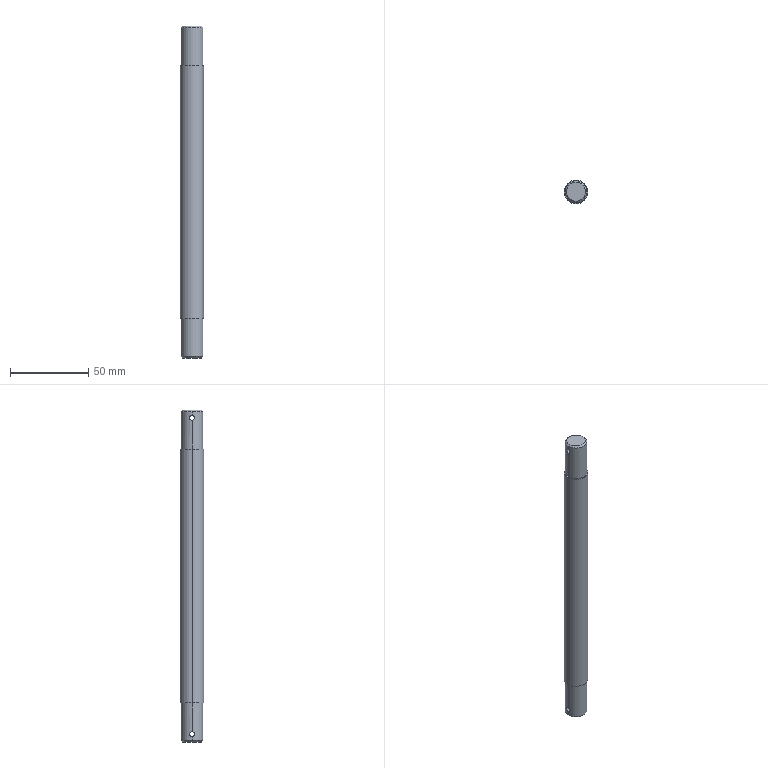Part | SolidWorks | features Chamfer 1, ICE 1, Revolution 1 | 1 solid | 18 faces | box 15 x 15 x 212 mm | volume 36086 mm3 | cylinder 10 | cone 4 | plane 4 | commonest cylinder face diameters 3 x4 14 x4 15 x2
STEP:
#1=CARTESIAN_POINT('',(6.,0.,0.));
#2=VERTEX_POINT('',#1);
#3=CARTESIAN_POINT('',(-6.,0.,0.));
#4=VERTEX_POINT('',#3);
#5=CARTESIAN_POINT('',(0.,0.,0.));
#6=DIRECTION('',(0.,0.,1.));
#7=DIRECTION('',(1.,0.,0.));
#8=AXIS2_PLACEMENT_3D('',#5,#6,#7);
#9=CIRCLE('',#8,6.);
#10=EDGE_CURVE('',#2,#4,#9,.T.);
#11=ORIENTED_EDGE('',*,*,#10,.F.);
#12=CARTESIAN_POINT('',(7.,0.,-1.));
#13=VERTEX_POINT('',#12);
#14=CARTESIAN_POINT('',(6.,0.,0.));
#15=DIRECTION('',(0.7071,0.,-0.7071));
#16=VECTOR('',#15,1000.);
#17=LINE('',#14,#16);
#18=EDGE_CURVE('',#2,#13,#17,.T.);
#19=ORIENTED_EDGE('',*,*,#18,.T.);
#20=CARTESIAN_POINT('',(-7.,0.,-1.));
#21=VERTEX_POINT('',#20);
#22=CARTESIAN_POINT('',(0.,0.,-1.));
#23=DIRECTION('',(0.,0.,-1.));
#24=DIRECTION('',(1.,0.,0.));
#25=AXIS2_PLACEMENT_3D('',#22,#23,#24);
#26=CIRCLE('',#25,7.);
#27=EDGE_CURVE('',#21,#13,#26,.T.);
#28=ORIENTED_EDGE('',*,*,#27,.F.);
#29=CARTESIAN_POINT('',(-6.,0.,0.));
#30=DIRECTION('',(-0.7071,0.,-0.7071));
#31=VECTOR('',#30,1000.);
#32=LINE('',#29,#31);
#33=EDGE_CURVE('',#4,#21,#32,.T.);
#34=ORIENTED_EDGE('',*,*,#33,.F.);
#35=EDGE_LOOP('',(#11,#19,#28,#34));
#36=FACE_OUTER_BOUND('',#35,.T.);
#37=CARTESIAN_POINT('',(0.,0.,0.));
#38=DIRECTION('',(0.,0.,-1.));
#39=DIRECTION('',(-1.,0.,0.));
#40=AXIS2_PLACEMENT_3D('',#37,#38,#39);
#41=CONICAL_SURFACE('',#40,6.,0.7854);
#42=ADVANCED_FACE('',(#36),#41,.T.);
#43=CARTESIAN_POINT('',(-6.,0.,-212.));
#44=VERTEX_POINT('',#43);
#45=CARTESIAN_POINT('',(6.,0.,-212.));
#46=VERTEX_POINT('',#45);
#47=CARTESIAN_POINT('',(0.,0.,-212.));
#48=DIRECTION('',(0.,0.,-1.));
#49=DIRECTION('',(1.,0.,0.));
#50=AXIS2_PLACEMENT_3D('',#47,#48,#49);
#51=CIRCLE('',#50,6.);
#52=EDGE_CURVE('',#44,#46,#51,.T.);
#53=ORIENTED_EDGE('',*,*,#52,.F.);
#54=CARTESIAN_POINT('',(-7.,0.,-211.));
#55=VERTEX_POINT('',#54);
#56=CARTESIAN_POINT('',(-7.,0.,-211.));
#57=DIRECTION('',(-0.7071,0.,0.7071));
#58=VECTOR('',#57,1000.);
#59=LINE('',#56,#58);
#60=EDGE_CURVE('',#44,#55,#59,.T.);
#61=ORIENTED_EDGE('',*,*,#60,.T.);
#62=CARTESIAN_POINT('',(7.,0.,-211.));
#63=VERTEX_POINT('',#62);
#64=CARTESIAN_POINT('',(0.,0.,-211.));
#65=DIRECTION('',(0.,0.,1.));
#66=DIRECTION('',(1.,0.,0.));
#67=AXIS2_PLACEMENT_3D('',#64,#65,#66);
#68=CIRCLE('',#67,7.);
#69=EDGE_CURVE('',#63,#55,#68,.T.);
#70=ORIENTED_EDGE('',*,*,#69,.F.);
#71=CARTESIAN_POINT('',(7.,0.,-211.));
#72=DIRECTION('',(0.7071,0.,0.7071));
#73=VECTOR('',#72,1000.);
#74=LINE('',#71,#73);
#75=EDGE_CURVE('',#46,#63,#74,.T.);
#76=ORIENTED_EDGE('',*,*,#75,.F.);
#77=EDGE_LOOP('',(#53,#61,#70,#76));
#78=FACE_OUTER_BOUND('',#77,.T.);
#79=CARTESIAN_POINT('',(0.,0.,-211.));
#80=DIRECTION('',(0.,0.,1.));
#81=DIRECTION('',(1.,0.,0.));
#82=AXIS2_PLACEMENT_3D('',#79,#80,#81);
#83=CONICAL_SURFACE('',#82,7.,0.7854);
#84=ADVANCED_FACE('',(#78),#83,.T.);
#85=CARTESIAN_POINT('',(-7.,0.,-208.5));
#86=VERTEX_POINT('',#85);
#87=CARTESIAN_POINT('',(-7.,0.,-205.5));
#88=VERTEX_POINT('',#87);
#89=CARTESIAN_POINT('',(-7.,0.,-208.5));
#90=CARTESIAN_POINT('',(-7.,-0.09942,-208.5));
#91=CARTESIAN_POINT('',(-6.998,-0.1971,-208.49));
#92=CARTESIAN_POINT('',(-6.99,-0.3892,-208.452));
#93=CARTESIAN_POINT('',(-6.984,-0.4847,-208.423));
#94=CARTESIAN_POINT('',(-6.969,-0.6662,-208.348));
#95=CARTESIAN_POINT('',(-6.96,-0.7523,-208.301));
#96=CARTESIAN_POINT('',(-6.94,-0.9151,-208.193));
#97=CARTESIAN_POINT('',(-6.93,-0.992,-208.129));
#98=CARTESIAN_POINT('',(-6.898,-1.199,-207.922));
#99=CARTESIAN_POINT('',(-6.877,-1.31,-207.755));
#100=CARTESIAN_POINT('',(-6.846,-1.46,-207.395));
#101=CARTESIAN_POINT('',(-6.837,-1.5,-207.197));
#102=CARTESIAN_POINT('',(-6.837,-1.5,-206.902));
#103=CARTESIAN_POINT('',(-6.84,-1.49,-206.803));
#104=CARTESIAN_POINT('',(-6.848,-1.452,-206.61));
#105=CARTESIAN_POINT('',(-6.854,-1.423,-206.516));
#106=CARTESIAN_POINT('',(-6.877,-1.31,-206.243));
#107=CARTESIAN_POINT('',(-6.898,-1.2,-206.078));
#108=CARTESIAN_POINT('',(-6.93,-0.9909,-205.87));
#109=CARTESIAN_POINT('',(-6.94,-0.9154,-205.808));
#110=CARTESIAN_POINT('',(-6.96,-0.7532,-205.699));
#111=CARTESIAN_POINT('',(-6.969,-0.6653,-205.652));
#112=CARTESIAN_POINT('',(-6.984,-0.4841,-205.577));
#113=CARTESIAN_POINT('',(-6.99,-0.3905,-205.548));
#114=CARTESIAN_POINT('',(-6.998,-0.1976,-205.51));
#115=CARTESIAN_POINT('',(-7.,-0.09806,-205.5));
#116=CARTESIAN_POINT('',(-7.,0.,-205.5));
#117=B_SPLINE_CURVE_WITH_KNOTS('',3,(#89,#90,#91,#92,#93,#94,#95,#96,#97,#98,#99,#100,#101,#102,#103,#104,#105,#106,#107,#108,#109,#110,#111,#112,#113,#114,#115,#116),.UNSPECIFIED.,.F.,.F.,(4,2,2,2,2,2,2,2,2,2,2,2,2,4),(0.,0.000294,0.0005879,0.0008819,0.001176,0.001764,0.002352,0.002646,0.00294,0.003528,0.003821,0.004115,0.004409,0.004703),.UNSPECIFIED.);
#118=EDGE_CURVE('',#86,#88,#117,.T.);
#119=ORIENTED_EDGE('',*,*,#118,.T.);
#120=CARTESIAN_POINT('',(7.,0.,-205.5));
#121=VERTEX_POINT('',#120);
#122=CARTESIAN_POINT('',(-7.5,0.,-205.5));
#123=DIRECTION('',(1.,0.,0.));
#124=VECTOR('',#123,1000.);
#125=LINE('',#122,#124);
#126=EDGE_CURVE('',#88,#121,#125,.T.);
#127=ORIENTED_EDGE('',*,*,#126,.T.);
#128=CARTESIAN_POINT('',(7.,0.,-208.5));
#129=VERTEX_POINT('',#128);
#130=CARTESIAN_POINT('',(7.,0.,-205.5));
#131=CARTESIAN_POINT('',(7.,-0.1961,-205.5));
#132=CARTESIAN_POINT('',(6.991,-0.394,-205.54));
#133=CARTESIAN_POINT('',(6.962,-0.7552,-205.689));
#134=CARTESIAN_POINT('',(6.94,-0.9218,-205.801));
#135=CARTESIAN_POINT('',(6.909,-1.129,-206.008));
#136=CARTESIAN_POINT('',(6.898,-1.192,-206.085));
#137=CARTESIAN_POINT('',(6.878,-1.301,-206.247));
#138=CARTESIAN_POINT('',(6.869,-1.347,-206.333));
#139=CARTESIAN_POINT('',(6.846,-1.461,-206.606));
#140=CARTESIAN_POINT('',(6.837,-1.5,-206.801));
#141=CARTESIAN_POINT('',(6.837,-1.5,-207.098));
#142=CARTESIAN_POINT('',(6.84,-1.49,-207.196));
#143=CARTESIAN_POINT('',(6.848,-1.452,-207.388));
#144=CARTESIAN_POINT('',(6.854,-1.423,-207.484));
#145=CARTESIAN_POINT('',(6.877,-1.311,-207.756));
#146=CARTESIAN_POINT('',(6.898,-1.199,-207.922));
#147=CARTESIAN_POINT('',(6.94,-0.9236,-208.198));
#148=CARTESIAN_POINT('',(6.961,-0.7569,-208.31));
#149=CARTESIAN_POINT('',(6.991,-0.396,-208.46));
#150=CARTESIAN_POINT('',(7.,-0.1988,-208.5));
#151=CARTESIAN_POINT('',(7.,0.,-208.5));
#152=B_SPLINE_CURVE_WITH_KNOTS('',3,(#130,#131,#132,#133,#134,#135,#136,#137,#138,#139,#140,#141,#142,#143,#144,#145,#146,#147,#148,#149,#150,#151),.UNSPECIFIED.,.F.,.F.,(4,2,2,2,2,2,2,2,2,2,4),(0.004703,0.005291,0.005879,0.006173,0.006467,0.007054,0.007348,0.007642,0.00823,0.008818,0.009405),.UNSPECIFIED.);
#153=EDGE_CURVE('',#121,#129,#152,.T.);
#154=ORIENTED_EDGE('',*,*,#153,.T.);
#155=CARTESIAN_POINT('',(-7.5,0.,-208.5));
#156=DIRECTION('',(1.,0.,0.));
#157=VECTOR('',#156,1000.);
#158=LINE('',#155,#157);
#159=EDGE_CURVE('',#86,#129,#158,.T.);
#160=ORIENTED_EDGE('',*,*,#159,.F.);
#161=EDGE_LOOP('',(#119,#127,#154,#160));
#162=FACE_OUTER_BOUND('',#161,.T.);
#163=CARTESIAN_POINT('',(-7.5,0.,-207.));
#164=DIRECTION('',(1.,0.,0.));
#165=DIRECTION('',(0.,0.,-1.));
#166=AXIS2_PLACEMENT_3D('',#163,#164,#165);
#167=CYLINDRICAL_SURFACE('',#166,1.5);
#168=ADVANCED_FACE('',(#162),#167,.F.);
#169=CARTESIAN_POINT('',(-7.,0.,-6.5));
#170=VERTEX_POINT('',#169);
#171=CARTESIAN_POINT('',(-7.,0.,-3.5));
#172=VERTEX_POINT('',#171);
#173=CARTESIAN_POINT('',(-7.,0.,-6.5));
#174=CARTESIAN_POINT('',(-7.,-0.09942,-6.5));
#175=CARTESIAN_POINT('',(-6.998,-0.1971,-6.49));
#176=CARTESIAN_POINT('',(-6.99,-0.3892,-6.452));
#177=CARTESIAN_POINT('',(-6.984,-0.4847,-6.423));
#178=CARTESIAN_POINT('',(-6.969,-0.6662,-6.348));
#179=CARTESIAN_POINT('',(-6.96,-0.7523,-6.301));
#180=CARTESIAN_POINT('',(-6.94,-0.9151,-6.193));
#181=CARTESIAN_POINT('',(-6.93,-0.992,-6.129));
#182=CARTESIAN_POINT('',(-6.898,-1.199,-5.922));
#183=CARTESIAN_POINT('',(-6.877,-1.31,-5.755));
#184=CARTESIAN_POINT('',(-6.846,-1.46,-5.395));
#185=CARTESIAN_POINT('',(-6.837,-1.5,-5.197));
#186=CARTESIAN_POINT('',(-6.837,-1.5,-4.902));
#187=CARTESIAN_POINT('',(-6.84,-1.49,-4.803));
#188=CARTESIAN_POINT('',(-6.848,-1.452,-4.61));
#189=CARTESIAN_POINT('',(-6.854,-1.423,-4.516));
#190=CARTESIAN_POINT('',(-6.877,-1.31,-4.243));
#191=CARTESIAN_POINT('',(-6.898,-1.2,-4.078));
#192=CARTESIAN_POINT('',(-6.93,-0.9909,-3.87));
#193=CARTESIAN_POINT('',(-6.94,-0.9154,-3.808));
#194=CARTESIAN_POINT('',(-6.96,-0.7532,-3.699));
#195=CARTESIAN_POINT('',(-6.969,-0.6653,-3.652));
#196=CARTESIAN_POINT('',(-6.984,-0.4841,-3.577));
#197=CARTESIAN_POINT('',(-6.99,-0.3905,-3.548));
#198=CARTESIAN_POINT('',(-6.998,-0.1976,-3.51));
#199=CARTESIAN_POINT('',(-7.,-0.09806,-3.5));
#200=CARTESIAN_POINT('',(-7.,0.,-3.5));
#201=B_SPLINE_CURVE_WITH_KNOTS('',3,(#173,#174,#175,#176,#177,#178,#179,#180,#181,#182,#183,#184,#185,#186,#187,#188,#189,#190,#191,#192,#193,#194,#195,#196,#197,#198,#199,#200),.UNSPECIFIED.,.F.,.F.,(4,2,2,2,2,2,2,2,2,2,2,2,2,4),(0.,0.000294,0.0005879,0.0008819,0.001176,0.001764,0.002352,0.002646,0.00294,0.003528,0.003821,0.004115,0.004409,0.004703),.UNSPECIFIED.);
#202=EDGE_CURVE('',#170,#172,#201,.T.);
#203=ORIENTED_EDGE('',*,*,#202,.T.);
#204=CARTESIAN_POINT('',(7.,0.,-3.5));
#205=VERTEX_POINT('',#204);
#206=CARTESIAN_POINT('',(-7.5,0.,-3.5));
#207=DIRECTION('',(1.,0.,0.));
#208=VECTOR('',#207,1000.);
#209=LINE('',#206,#208);
#210=EDGE_CURVE('',#172,#205,#209,.T.);
#211=ORIENTED_EDGE('',*,*,#210,.T.);
#212=CARTESIAN_POINT('',(7.,0.,-6.5));
#213=VERTEX_POINT('',#212);
#214=CARTESIAN_POINT('',(7.,0.,-3.5));
#215=CARTESIAN_POINT('',(7.,-0.1961,-3.5));
#216=CARTESIAN_POINT('',(6.991,-0.394,-3.54));
#217=CARTESIAN_POINT('',(6.962,-0.7552,-3.689));
#218=CARTESIAN_POINT('',(6.94,-0.9218,-3.801));
#219=CARTESIAN_POINT('',(6.909,-1.129,-4.008));
#220=CARTESIAN_POINT('',(6.898,-1.192,-4.085));
#221=CARTESIAN_POINT('',(6.878,-1.301,-4.247));
#222=CARTESIAN_POINT('',(6.869,-1.347,-4.333));
#223=CARTESIAN_POINT('',(6.846,-1.461,-4.606));
#224=CARTESIAN_POINT('',(6.837,-1.5,-4.801));
#225=CARTESIAN_POINT('',(6.837,-1.5,-5.098));
#226=CARTESIAN_POINT('',(6.84,-1.49,-5.196));
#227=CARTESIAN_POINT('',(6.848,-1.452,-5.388));
#228=CARTESIAN_POINT('',(6.854,-1.423,-5.484));
#229=CARTESIAN_POINT('',(6.877,-1.311,-5.756));
#230=CARTESIAN_POINT('',(6.898,-1.199,-5.922));
#231=CARTESIAN_POINT('',(6.94,-0.9236,-6.198));
#232=CARTESIAN_POINT('',(6.961,-0.7569,-6.31));
#233=CARTESIAN_POINT('',(6.991,-0.396,-6.46));
#234=CARTESIAN_POINT('',(7.,-0.1988,-6.5));
#235=CARTESIAN_POINT('',(7.,0.,-6.5));
#236=B_SPLINE_CURVE_WITH_KNOTS('',3,(#214,#215,#216,#217,#218,#219,#220,#221,#222,#223,#224,#225,#226,#227,#228,#229,#230,#231,#232,#233,#234,#235),.UNSPECIFIED.,.F.,.F.,(4,2,2,2,2,2,2,2,2,2,4),(0.004703,0.005291,0.005879,0.006173,0.006467,0.007054,0.007348,0.007642,0.00823,0.008818,0.009405),.UNSPECIFIED.);
#237=EDGE_CURVE('',#205,#213,#236,.T.);
#238=ORIENTED_EDGE('',*,*,#237,.T.);
#239=CARTESIAN_POINT('',(-7.5,0.,-6.5));
#240=DIRECTION('',(1.,0.,0.));
#241=VECTOR('',#240,1000.);
#242=LINE('',#239,#241);
#243=EDGE_CURVE('',#170,#213,#242,.T.);
#244=ORIENTED_EDGE('',*,*,#243,.F.);
#245=EDGE_LOOP('',(#203,#211,#238,#244));
#246=FACE_OUTER_BOUND('',#245,.T.);
#247=CARTESIAN_POINT('',(-7.5,0.,-5.));
#248=DIRECTION('',(1.,0.,0.));
#249=DIRECTION('',(0.,0.,-1.));
#250=AXIS2_PLACEMENT_3D('',#247,#248,#249);
#251=CYLINDRICAL_SURFACE('',#250,1.5);
#252=ADVANCED_FACE('',(#246),#251,.F.);
#253=CARTESIAN_POINT('',(7.,0.,-25.));
#254=VERTEX_POINT('',#253);
#255=CARTESIAN_POINT('',(-7.,0.,-25.));
#256=VERTEX_POINT('',#255);
#257=CARTESIAN_POINT('',(0.,0.,-25.));
#258=DIRECTION('',(0.,0.,1.));
#259=DIRECTION('',(1.,0.,0.));
#260=AXIS2_PLACEMENT_3D('',#257,#258,#259);
#261=CIRCLE('',#260,7.);
#262=EDGE_CURVE('',#254,#256,#261,.T.);
#263=ORIENTED_EDGE('',*,*,#262,.T.);
#264=CARTESIAN_POINT('',(-7.,0.,-25.));
#265=DIRECTION('',(0.,0.,1.));
#266=VECTOR('',#265,1000.);
#267=LINE('',#264,#266);
#268=EDGE_CURVE('',#256,#170,#267,.T.);
#269=ORIENTED_EDGE('',*,*,#268,.T.);
#270=CARTESIAN_POINT('',(-7.,0.,-3.5));
#271=CARTESIAN_POINT('',(-7.,0.1961,-3.5));
#272=CARTESIAN_POINT('',(-6.991,0.394,-3.54));
#273=CARTESIAN_POINT('',(-6.962,0.7552,-3.689));
#274=CARTESIAN_POINT('',(-6.94,0.9218,-3.801));
#275=CARTESIAN_POINT('',(-6.909,1.129,-4.008));
#276=CARTESIAN_POINT('',(-6.898,1.192,-4.085));
#277=CARTESIAN_POINT('',(-6.878,1.301,-4.247));
#278=CARTESIAN_POINT('',(-6.869,1.347,-4.333));
#279=CARTESIAN_POINT('',(-6.846,1.461,-4.606));
#280=CARTESIAN_POINT('',(-6.837,1.5,-4.801));
#281=CARTESIAN_POINT('',(-6.837,1.5,-5.098));
#282=CARTESIAN_POINT('',(-6.84,1.49,-5.196));
#283=CARTESIAN_POINT('',(-6.848,1.452,-5.388));
#284=CARTESIAN_POINT('',(-6.854,1.423,-5.484));
#285=CARTESIAN_POINT('',(-6.877,1.311,-5.756));
#286=CARTESIAN_POINT('',(-6.898,1.199,-5.922));
#287=CARTESIAN_POINT('',(-6.94,0.9236,-6.198));
#288=CARTESIAN_POINT('',(-6.961,0.7569,-6.31));
#289=CARTESIAN_POINT('',(-6.991,0.396,-6.46));
#290=CARTESIAN_POINT('',(-7.,0.1988,-6.5));
#291=CARTESIAN_POINT('',(-7.,0.,-6.5));
#292=B_SPLINE_CURVE_WITH_KNOTS('',3,(#270,#271,#272,#273,#274,#275,#276,#277,#278,#279,#280,#281,#282,#283,#284,#285,#286,#287,#288,#289,#290,#291),.UNSPECIFIED.,.F.,.F.,(4,2,2,2,2,2,2,2,2,2,4),(0.004703,0.005291,0.005879,0.006173,0.006467,0.007054,0.007348,0.007642,0.00823,0.008818,0.009405),.UNSPECIFIED.);
#293=EDGE_CURVE('',#172,#170,#292,.T.);
#294=ORIENTED_EDGE('',*,*,#293,.F.);
#295=CARTESIAN_POINT('',(-7.,0.,-25.));
#296=DIRECTION('',(0.,0.,1.));
#297=VECTOR('',#296,1000.);
#298=LINE('',#295,#297);
#299=EDGE_CURVE('',#172,#21,#298,.T.);
#300=ORIENTED_EDGE('',*,*,#299,.T.);
#301=ORIENTED_EDGE('',*,*,#27,.T.);
#302=CARTESIAN_POINT('',(7.,0.,-25.));
#303=DIRECTION('',(0.,0.,1.));
#304=VECTOR('',#303,1000.);
#305=LINE('',#302,#304);
#306=EDGE_CURVE('',#205,#13,#305,.T.);
#307=ORIENTED_EDGE('',*,*,#306,.F.);
#308=CARTESIAN_POINT('',(7.,0.,-6.5));
#309=CARTESIAN_POINT('',(7.,0.09942,-6.5));
#310=CARTESIAN_POINT('',(6.998,0.1971,-6.49));
#311=CARTESIAN_POINT('',(6.99,0.3892,-6.452));
#312=CARTESIAN_POINT('',(6.984,0.4847,-6.423));
#313=CARTESIAN_POINT('',(6.969,0.6662,-6.348));
#314=CARTESIAN_POINT('',(6.96,0.7523,-6.301));
#315=CARTESIAN_POINT('',(6.94,0.9151,-6.193));
#316=CARTESIAN_POINT('',(6.93,0.992,-6.129));
#317=CARTESIAN_POINT('',(6.898,1.199,-5.922));
#318=CARTESIAN_POINT('',(6.877,1.31,-5.755));
#319=CARTESIAN_POINT('',(6.846,1.46,-5.395));
#320=CARTESIAN_POINT('',(6.837,1.5,-5.197));
#321=CARTESIAN_POINT('',(6.837,1.5,-4.902));
#322=CARTESIAN_POINT('',(6.84,1.49,-4.803));
#323=CARTESIAN_POINT('',(6.848,1.452,-4.61));
#324=CARTESIAN_POINT('',(6.854,1.423,-4.516));
#325=CARTESIAN_POINT('',(6.877,1.31,-4.243));
#326=CARTESIAN_POINT('',(6.898,1.2,-4.078));
#327=CARTESIAN_POINT('',(6.93,0.9909,-3.87));
#328=CARTESIAN_POINT('',(6.94,0.9154,-3.808));
#329=CARTESIAN_POINT('',(6.96,0.7532,-3.699));
#330=CARTESIAN_POINT('',(6.969,0.6653,-3.652));
#331=CARTESIAN_POINT('',(6.984,0.4841,-3.577));
#332=CARTESIAN_POINT('',(6.99,0.3905,-3.548));
#333=CARTESIAN_POINT('',(6.998,0.1976,-3.51));
#334=CARTESIAN_POINT('',(7.,0.09806,-3.5));
#335=CARTESIAN_POINT('',(7.,0.,-3.5));
#336=B_SPLINE_CURVE_WITH_KNOTS('',3,(#308,#309,#310,#311,#312,#313,#314,#315,#316,#317,#318,#319,#320,#321,#322,#323,#324,#325,#326,#327,#328,#329,#330,#331,#332,#333,#334,#335),.UNSPECIFIED.,.F.,.F.,(4,2,2,2,2,2,2,2,2,2,2,2,2,4),(0.,0.000294,0.0005879,0.0008819,0.001176,0.001764,0.002352,0.002646,0.00294,0.003528,0.003821,0.004115,0.004409,0.004703),.UNSPECIFIED.);
#337=EDGE_CURVE('',#213,#205,#336,.T.);
#338=ORIENTED_EDGE('',*,*,#337,.F.);
#339=CARTESIAN_POINT('',(7.,0.,-25.));
#340=DIRECTION('',(0.,0.,1.));
#341=VECTOR('',#340,1000.);
#342=LINE('',#339,#341);
#343=EDGE_CURVE('',#254,#213,#342,.T.);
#344=ORIENTED_EDGE('',*,*,#343,.F.);
#345=EDGE_LOOP('',(#263,#269,#294,#300,#301,#307,#338,#344));
#346=FACE_OUTER_BOUND('',#345,.T.);
#347=CARTESIAN_POINT('',(0.,0.,-25.));
#348=DIRECTION('',(0.,0.,1.));
#349=DIRECTION('',(1.,0.,0.));
#350=AXIS2_PLACEMENT_3D('',#347,#348,#349);
#351=CYLINDRICAL_SURFACE('',#350,7.);
#352=ADVANCED_FACE('',(#346),#351,.T.);
#353=CARTESIAN_POINT('',(7.5,0.,-187.));
#354=VERTEX_POINT('',#353);
#355=CARTESIAN_POINT('',(-7.5,0.,-187.));
#356=VERTEX_POINT('',#355);
#357=CARTESIAN_POINT('',(0.,0.,-187.));
#358=DIRECTION('',(0.,0.,1.));
#359=DIRECTION('',(1.,0.,0.));
#360=AXIS2_PLACEMENT_3D('',#357,#358,#359);
#361=CIRCLE('',#360,7.5);
#362=EDGE_CURVE('',#354,#356,#361,.T.);
#363=ORIENTED_EDGE('',*,*,#362,.T.);
#364=CARTESIAN_POINT('',(-7.5,0.,-25.));
#365=VERTEX_POINT('',#364);
#366=CARTESIAN_POINT('',(-7.5,0.,-25.));
#367=DIRECTION('',(0.,0.,1.));
#368=VECTOR('',#367,1000.);
#369=LINE('',#366,#368);
#370=EDGE_CURVE('',#356,#365,#369,.T.);
#371=ORIENTED_EDGE('',*,*,#370,.T.);
#372=CARTESIAN_POINT('',(7.5,0.,-25.));
#373=VERTEX_POINT('',#372);
#374=CARTESIAN_POINT('',(0.,0.,-25.));
#375=DIRECTION('',(0.,0.,1.));
#376=DIRECTION('',(1.,0.,0.));
#377=AXIS2_PLACEMENT_3D('',#374,#375,#376);
#378=CIRCLE('',#377,7.5);
#379=EDGE_CURVE('',#373,#365,#378,.T.);
#380=ORIENTED_EDGE('',*,*,#379,.F.);
#381=CARTESIAN_POINT('',(7.5,0.,-25.));
#382=DIRECTION('',(0.,0.,1.));
#383=VECTOR('',#382,1000.);
#384=LINE('',#381,#383);
#385=EDGE_CURVE('',#354,#373,#384,.T.);
#386=ORIENTED_EDGE('',*,*,#385,.F.);
#387=EDGE_LOOP('',(#363,#371,#380,#386));
#388=FACE_OUTER_BOUND('',#387,.T.);
#389=CARTESIAN_POINT('',(0.,0.,-25.));
#390=DIRECTION('',(0.,0.,1.));
#391=DIRECTION('',(1.,0.,0.));
#392=AXIS2_PLACEMENT_3D('',#389,#390,#391);
#393=CYLINDRICAL_SURFACE('',#392,7.5);
#394=ADVANCED_FACE('',(#388),#393,.T.);
#395=ORIENTED_EDGE('',*,*,#69,.T.);
#396=CARTESIAN_POINT('',(-7.,0.,-25.));
#397=DIRECTION('',(0.,0.,1.));
#398=VECTOR('',#397,1000.);
#399=LINE('',#396,#398);
#400=EDGE_CURVE('',#55,#86,#399,.T.);
#401=ORIENTED_EDGE('',*,*,#400,.T.);
#402=CARTESIAN_POINT('',(-7.,0.,-205.5));
#403=CARTESIAN_POINT('',(-7.,0.1961,-205.5));
#404=CARTESIAN_POINT('',(-6.991,0.394,-205.54));
#405=CARTESIAN_POINT('',(-6.962,0.7552,-205.689));
#406=CARTESIAN_POINT('',(-6.94,0.9218,-205.801));
#407=CARTESIAN_POINT('',(-6.909,1.129,-206.008));
#408=CARTESIAN_POINT('',(-6.898,1.192,-206.085));
#409=CARTESIAN_POINT('',(-6.878,1.301,-206.247));
#410=CARTESIAN_POINT('',(-6.869,1.347,-206.333));
#411=CARTESIAN_POINT('',(-6.846,1.461,-206.606));
#412=CARTESIAN_POINT('',(-6.837,1.5,-206.801));
#413=CARTESIAN_POINT('',(-6.837,1.5,-207.098));
#414=CARTESIAN_POINT('',(-6.84,1.49,-207.196));
#415=CARTESIAN_POINT('',(-6.848,1.452,-207.388));
#416=CARTESIAN_POINT('',(-6.854,1.423,-207.484));
#417=CARTESIAN_POINT('',(-6.877,1.311,-207.756));
#418=CARTESIAN_POINT('',(-6.898,1.199,-207.922));
#419=CARTESIAN_POINT('',(-6.94,0.9236,-208.198));
#420=CARTESIAN_POINT('',(-6.961,0.7569,-208.31));
#421=CARTESIAN_POINT('',(-6.991,0.396,-208.46));
#422=CARTESIAN_POINT('',(-7.,0.1988,-208.5));
#423=CARTESIAN_POINT('',(-7.,0.,-208.5));
#424=B_SPLINE_CURVE_WITH_KNOTS('',3,(#402,#403,#404,#405,#406,#407,#408,#409,#410,#411,#412,#413,#414,#415,#416,#417,#418,#419,#420,#421,#422,#423),.UNSPECIFIED.,.F.,.F.,(4,2,2,2,2,2,2,2,2,2,4),(0.004703,0.005291,0.005879,0.006173,0.006467,0.007054,0.007348,0.007642,0.00823,0.008818,0.009405),.UNSPECIFIED.);
#425=EDGE_CURVE('',#88,#86,#424,.T.);
#426=ORIENTED_EDGE('',*,*,#425,.F.);
#427=CARTESIAN_POINT('',(-7.,0.,-187.));
#428=VERTEX_POINT('',#427);
#429=CARTESIAN_POINT('',(-7.,0.,-25.));
#430=DIRECTION('',(0.,0.,1.));
#431=VECTOR('',#430,1000.);
#432=LINE('',#429,#431);
#433=EDGE_CURVE('',#88,#428,#432,.T.);
#434=ORIENTED_EDGE('',*,*,#433,.T.);
#435=CARTESIAN_POINT('',(7.,0.,-187.));
#436=VERTEX_POINT('',#435);
#437=CARTESIAN_POINT('',(0.,0.,-187.));
#438=DIRECTION('',(0.,0.,1.));
#439=DIRECTION('',(1.,0.,0.));
#440=AXIS2_PLACEMENT_3D('',#437,#438,#439);
#441=CIRCLE('',#440,7.);
#442=EDGE_CURVE('',#436,#428,#441,.T.);
#443=ORIENTED_EDGE('',*,*,#442,.F.);
#444=CARTESIAN_POINT('',(7.,0.,-25.));
#445=DIRECTION('',(0.,0.,1.));
#446=VECTOR('',#445,1000.);
#447=LINE('',#444,#446);
#448=EDGE_CURVE('',#121,#436,#447,.T.);
#449=ORIENTED_EDGE('',*,*,#448,.F.);
#450=CARTESIAN_POINT('',(7.,0.,-208.5));
#451=CARTESIAN_POINT('',(7.,0.09942,-208.5));
#452=CARTESIAN_POINT('',(6.998,0.1971,-208.49));
#453=CARTESIAN_POINT('',(6.99,0.3892,-208.452));
#454=CARTESIAN_POINT('',(6.984,0.4847,-208.423));
#455=CARTESIAN_POINT('',(6.969,0.6662,-208.348));
#456=CARTESIAN_POINT('',(6.96,0.7523,-208.301));
#457=CARTESIAN_POINT('',(6.94,0.9151,-208.193));
#458=CARTESIAN_POINT('',(6.93,0.992,-208.129));
#459=CARTESIAN_POINT('',(6.898,1.199,-207.922));
#460=CARTESIAN_POINT('',(6.877,1.31,-207.755));
#461=CARTESIAN_POINT('',(6.846,1.46,-207.395));
#462=CARTESIAN_POINT('',(6.837,1.5,-207.197));
#463=CARTESIAN_POINT('',(6.837,1.5,-206.902));
#464=CARTESIAN_POINT('',(6.84,1.49,-206.803));
#465=CARTESIAN_POINT('',(6.848,1.452,-206.61));
#466=CARTESIAN_POINT('',(6.854,1.423,-206.516));
#467=CARTESIAN_POINT('',(6.877,1.31,-206.243));
#468=CARTESIAN_POINT('',(6.898,1.2,-206.078));
#469=CARTESIAN_POINT('',(6.93,0.9909,-205.87));
#470=CARTESIAN_POINT('',(6.94,0.9154,-205.808));
#471=CARTESIAN_POINT('',(6.96,0.7532,-205.699));
#472=CARTESIAN_POINT('',(6.969,0.6653,-205.652));
#473=CARTESIAN_POINT('',(6.984,0.4841,-205.577));
#474=CARTESIAN_POINT('',(6.99,0.3905,-205.548));
#475=CARTESIAN_POINT('',(6.998,0.1976,-205.51));
#476=CARTESIAN_POINT('',(7.,0.09806,-205.5));
#477=CARTESIAN_POINT('',(7.,0.,-205.5));
#478=B_SPLINE_CURVE_WITH_KNOTS('',3,(#450,#451,#452,#453,#454,#455,#456,#457,#458,#459,#460,#461,#462,#463,#464,#465,#466,#467,#468,#469,#470,#471,#472,#473,#474,#475,#476,#477),.UNSPECIFIED.,.F.,.F.,(4,2,2,2,2,2,2,2,2,2,2,2,2,4),(0.,0.000294,0.0005879,0.0008819,0.001176,0.001764,0.002352,0.002646,0.00294,0.003528,0.003821,0.004115,0.004409,0.004703),.UNSPECIFIED.);
#479=EDGE_CURVE('',#129,#121,#478,.T.);
#480=ORIENTED_EDGE('',*,*,#479,.F.);
#481=CARTESIAN_POINT('',(7.,0.,-25.));
#482=DIRECTION('',(0.,0.,1.));
#483=VECTOR('',#482,1000.);
#484=LINE('',#481,#483);
#485=EDGE_CURVE('',#63,#129,#484,.T.);
#486=ORIENTED_EDGE('',*,*,#485,.F.);
#487=EDGE_LOOP('',(#395,#401,#426,#434,#443,#449,#480,#486));
#488=FACE_OUTER_BOUND('',#487,.T.);
#489=CARTESIAN_POINT('',(0.,0.,-25.));
#490=DIRECTION('',(0.,0.,1.));
#491=DIRECTION('',(1.,0.,0.));
#492=AXIS2_PLACEMENT_3D('',#489,#490,#491);
#493=CYLINDRICAL_SURFACE('',#492,7.);
#494=ADVANCED_FACE('',(#488),#493,.T.);
#495=CARTESIAN_POINT('',(0.,0.,-212.));
#496=DIRECTION('',(0.,0.,-1.));
#497=DIRECTION('',(1.,0.,0.));
#498=AXIS2_PLACEMENT_3D('',#495,#496,#497);
#499=CIRCLE('',#498,6.);
#500=EDGE_CURVE('',#46,#44,#499,.T.);
#501=ORIENTED_EDGE('',*,*,#500,.T.);
#502=ORIENTED_EDGE('',*,*,#52,.T.);
#503=EDGE_LOOP('',(#501,#502));
#504=FACE_OUTER_BOUND('',#503,.T.);
#505=CARTESIAN_POINT('',(0.,0.,-212.));
#506=DIRECTION('',(0.,0.,1.));
#507=DIRECTION('',(1.,0.,0.));
#508=AXIS2_PLACEMENT_3D('',#505,#506,#507);
#509=PLANE('',#508);
#510=ADVANCED_FACE('',(#504),#509,.F.);
#511=ORIENTED_EDGE('',*,*,#400,.F.);
#512=CARTESIAN_POINT('',(0.,0.,-211.));
#513=DIRECTION('',(0.,0.,1.));
#514=DIRECTION('',(1.,0.,0.));
#515=AXIS2_PLACEMENT_3D('',#512,#513,#514);
#516=CIRCLE('',#515,7.);
#517=EDGE_CURVE('',#55,#63,#516,.T.);
#518=ORIENTED_EDGE('',*,*,#517,.T.);
#519=ORIENTED_EDGE('',*,*,#485,.T.);
#520=ORIENTED_EDGE('',*,*,#153,.F.);
#521=ORIENTED_EDGE('',*,*,#448,.T.);
#522=CARTESIAN_POINT('',(0.,0.,-187.));
#523=DIRECTION('',(0.,0.,1.));
#524=DIRECTION('',(1.,0.,0.));
#525=AXIS2_PLACEMENT_3D('',#522,#523,#524);
#526=CIRCLE('',#525,7.);
#527=EDGE_CURVE('',#428,#436,#526,.T.);
#528=ORIENTED_EDGE('',*,*,#527,.F.);
#529=ORIENTED_EDGE('',*,*,#433,.F.);
#530=ORIENTED_EDGE('',*,*,#118,.F.);
#531=EDGE_LOOP('',(#511,#518,#519,#520,#521,#528,#529,#530));
#532=FACE_OUTER_BOUND('',#531,.T.);
#533=CARTESIAN_POINT('',(0.,0.,-25.));
#534=DIRECTION('',(0.,0.,1.));
#535=DIRECTION('',(1.,0.,0.));
#536=AXIS2_PLACEMENT_3D('',#533,#534,#535);
#537=CYLINDRICAL_SURFACE('',#536,7.);
#538=ADVANCED_FACE('',(#532),#537,.T.);
#539=ORIENTED_EDGE('',*,*,#362,.F.);
#540=CARTESIAN_POINT('',(0.,0.,-187.));
#541=DIRECTION('',(0.,0.,1.));
#542=DIRECTION('',(1.,0.,0.));
#543=AXIS2_PLACEMENT_3D('',#540,#541,#542);
#544=CIRCLE('',#543,7.5);
#545=EDGE_CURVE('',#356,#354,#544,.T.);
#546=ORIENTED_EDGE('',*,*,#545,.F.);
#547=EDGE_LOOP('',(#539,#546));
#548=FACE_OUTER_BOUND('',#547,.T.);
#549=ORIENTED_EDGE('',*,*,#442,.T.);
#550=ORIENTED_EDGE('',*,*,#527,.T.);
#551=EDGE_LOOP('',(#549,#550));
#552=FACE_BOUND('',#551,.T.);
#553=CARTESIAN_POINT('',(0.,0.,-187.));
#554=DIRECTION('',(0.,0.,1.));
#555=DIRECTION('',(1.,0.,0.));
#556=AXIS2_PLACEMENT_3D('',#553,#554,#555);
#557=PLANE('',#556);
#558=ADVANCED_FACE('',(#548,#552),#557,.F.);
#559=ORIENTED_EDGE('',*,*,#370,.F.);
#560=ORIENTED_EDGE('',*,*,#545,.T.);
#561=ORIENTED_EDGE('',*,*,#385,.T.);
#562=CARTESIAN_POINT('',(0.,0.,-25.));
#563=DIRECTION('',(0.,0.,1.));
#564=DIRECTION('',(1.,0.,0.));
#565=AXIS2_PLACEMENT_3D('',#562,#563,#564);
#566=CIRCLE('',#565,7.5);
#567=EDGE_CURVE('',#365,#373,#566,.T.);
#568=ORIENTED_EDGE('',*,*,#567,.F.);
#569=EDGE_LOOP('',(#559,#560,#561,#568));
#570=FACE_OUTER_BOUND('',#569,.T.);
#571=CARTESIAN_POINT('',(0.,0.,-25.));
#572=DIRECTION('',(0.,0.,1.));
#573=DIRECTION('',(1.,0.,0.));
#574=AXIS2_PLACEMENT_3D('',#571,#572,#573);
#575=CYLINDRICAL_SURFACE('',#574,7.5);
#576=ADVANCED_FACE('',(#570),#575,.T.);
#577=ORIENTED_EDGE('',*,*,#379,.T.);
#578=ORIENTED_EDGE('',*,*,#567,.T.);
#579=EDGE_LOOP('',(#577,#578));
#580=FACE_OUTER_BOUND('',#579,.T.);
#581=ORIENTED_EDGE('',*,*,#262,.F.);
#582=CARTESIAN_POINT('',(0.,0.,-25.));
#583=DIRECTION('',(0.,0.,1.));
#584=DIRECTION('',(1.,0.,0.));
#585=AXIS2_PLACEMENT_3D('',#582,#583,#584);
#586=CIRCLE('',#585,7.);
#587=EDGE_CURVE('',#256,#254,#586,.T.);
#588=ORIENTED_EDGE('',*,*,#587,.F.);
#589=EDGE_LOOP('',(#581,#588));
#590=FACE_BOUND('',#589,.T.);
#591=CARTESIAN_POINT('',(0.,0.,-25.));
#592=DIRECTION('',(0.,0.,1.));
#593=DIRECTION('',(1.,0.,0.));
#594=AXIS2_PLACEMENT_3D('',#591,#592,#593);
#595=PLANE('',#594);
#596=ADVANCED_FACE('',(#580,#590),#595,.T.);
#597=ORIENTED_EDGE('',*,*,#268,.F.);
#598=ORIENTED_EDGE('',*,*,#587,.T.);
#599=ORIENTED_EDGE('',*,*,#343,.T.);
#600=ORIENTED_EDGE('',*,*,#237,.F.);
#601=ORIENTED_EDGE('',*,*,#306,.T.);
#602=CARTESIAN_POINT('',(0.,0.,-1.));
#603=DIRECTION('',(0.,0.,-1.));
#604=DIRECTION('',(1.,0.,0.));
#605=AXIS2_PLACEMENT_3D('',#602,#603,#604);
#606=CIRCLE('',#605,7.);
#607=EDGE_CURVE('',#13,#21,#606,.T.);
#608=ORIENTED_EDGE('',*,*,#607,.T.);
#609=ORIENTED_EDGE('',*,*,#299,.F.);
#610=ORIENTED_EDGE('',*,*,#202,.F.);
#611=EDGE_LOOP('',(#597,#598,#599,#600,#601,#608,#609,#610));
#612=FACE_OUTER_BOUND('',#611,.T.);
#613=CARTESIAN_POINT('',(0.,0.,-25.));
#614=DIRECTION('',(0.,0.,1.));
#615=DIRECTION('',(1.,0.,0.));
#616=AXIS2_PLACEMENT_3D('',#613,#614,#615);
#617=CYLINDRICAL_SURFACE('',#616,7.);
#618=ADVANCED_FACE('',(#612),#617,.T.);
#619=CARTESIAN_POINT('',(0.,0.,0.));
#620=DIRECTION('',(0.,0.,1.));
#621=DIRECTION('',(1.,0.,0.));
#622=AXIS2_PLACEMENT_3D('',#619,#620,#621);
#623=CIRCLE('',#622,6.);
#624=EDGE_CURVE('',#4,#2,#623,.T.);
#625=ORIENTED_EDGE('',*,*,#624,.T.);
#626=ORIENTED_EDGE('',*,*,#10,.T.);
#627=EDGE_LOOP('',(#625,#626));
#628=FACE_OUTER_BOUND('',#627,.T.);
#629=CARTESIAN_POINT('',(0.,0.,0.));
#630=DIRECTION('',(0.,0.,1.));
#631=DIRECTION('',(1.,0.,0.));
#632=AXIS2_PLACEMENT_3D('',#629,#630,#631);
#633=PLANE('',#632);
#634=ADVANCED_FACE('',(#628),#633,.T.);
#635=ORIENTED_EDGE('',*,*,#210,.F.);
#636=ORIENTED_EDGE('',*,*,#293,.T.);
#637=ORIENTED_EDGE('',*,*,#243,.T.);
#638=ORIENTED_EDGE('',*,*,#337,.T.);
#639=EDGE_LOOP('',(#635,#636,#637,#638));
#640=FACE_OUTER_BOUND('',#639,.T.);
#641=CARTESIAN_POINT('',(-7.5,0.,-5.));
#642=DIRECTION('',(1.,0.,0.));
#643=DIRECTION('',(0.,0.,-1.));
#644=AXIS2_PLACEMENT_3D('',#641,#642,#643);
#645=CYLINDRICAL_SURFACE('',#644,1.5);
#646=ADVANCED_FACE('',(#640),#645,.F.);
#647=ORIENTED_EDGE('',*,*,#126,.F.);
#648=ORIENTED_EDGE('',*,*,#425,.T.);
#649=ORIENTED_EDGE('',*,*,#159,.T.);
#650=ORIENTED_EDGE('',*,*,#479,.T.);
#651=EDGE_LOOP('',(#647,#648,#649,#650));
#652=FACE_OUTER_BOUND('',#651,.T.);
#653=CARTESIAN_POINT('',(-7.5,0.,-207.));
#654=DIRECTION('',(1.,0.,0.));
#655=DIRECTION('',(0.,0.,-1.));
#656=AXIS2_PLACEMENT_3D('',#653,#654,#655);
#657=CYLINDRICAL_SURFACE('',#656,1.5);
#658=ADVANCED_FACE('',(#652),#657,.F.);
#659=ORIENTED_EDGE('',*,*,#60,.F.);
#660=ORIENTED_EDGE('',*,*,#500,.F.);
#661=ORIENTED_EDGE('',*,*,#75,.T.);
#662=ORIENTED_EDGE('',*,*,#517,.F.);
#663=EDGE_LOOP('',(#659,#660,#661,#662));
#664=FACE_OUTER_BOUND('',#663,.T.);
#665=CARTESIAN_POINT('',(0.,0.,-211.));
#666=DIRECTION('',(0.,0.,1.));
#667=DIRECTION('',(1.,0.,0.));
#668=AXIS2_PLACEMENT_3D('',#665,#666,#667);
#669=CONICAL_SURFACE('',#668,7.,0.7854);
#670=ADVANCED_FACE('',(#664),#669,.T.);
#671=ORIENTED_EDGE('',*,*,#18,.F.);
#672=ORIENTED_EDGE('',*,*,#624,.F.);
#673=ORIENTED_EDGE('',*,*,#33,.T.);
#674=ORIENTED_EDGE('',*,*,#607,.F.);
#675=EDGE_LOOP('',(#671,#672,#673,#674));
#676=FACE_OUTER_BOUND('',#675,.T.);
#677=CARTESIAN_POINT('',(0.,0.,0.));
#678=DIRECTION('',(0.,0.,-1.));
#679=DIRECTION('',(-1.,0.,0.));
#680=AXIS2_PLACEMENT_3D('',#677,#678,#679);
#681=CONICAL_SURFACE('',#680,6.,0.7854);
#682=ADVANCED_FACE('',(#676),#681,.T.);
#683=CLOSED_SHELL('',(#42,#84,#168,#252,#352,#394,#494,#510,#538,#558,#576,#596,#618,#634,#646,#658,#670,#682));
#684=MANIFOLD_SOLID_BREP('',#683);
#685=CARTESIAN_POINT('',(0.,0.,0.));
#686=DIRECTION('',(0.,0.,1.));
#687=DIRECTION('',(1.,0.,0.));
#688=AXIS2_PLACEMENT_3D('',#685,#686,#687);
#689=(LENGTH_UNIT()NAMED_UNIT(*)SI_UNIT(.MILLI.,.METRE.));
#690=UNCERTAINTY_MEASURE_WITH_UNIT(LENGTH_MEASURE(0.00001),#689,'','');
#691=(NAMED_UNIT(*)PLANE_ANGLE_UNIT()SI_UNIT($,.RADIAN.));
#692=(NAMED_UNIT(*)SI_UNIT($,.STERADIAN.)SOLID_ANGLE_UNIT());
#693=(GEOMETRIC_REPRESENTATION_CONTEXT(3)GLOBAL_UNCERTAINTY_ASSIGNED_CONTEXT((#690))GLOBAL_UNIT_ASSIGNED_CONTEXT((#689,#691,#692))REPRESENTATION_CONTEXT('',''));
#694=ADVANCED_BREP_SHAPE_REPRESENTATION('',(#684,#688),#693);